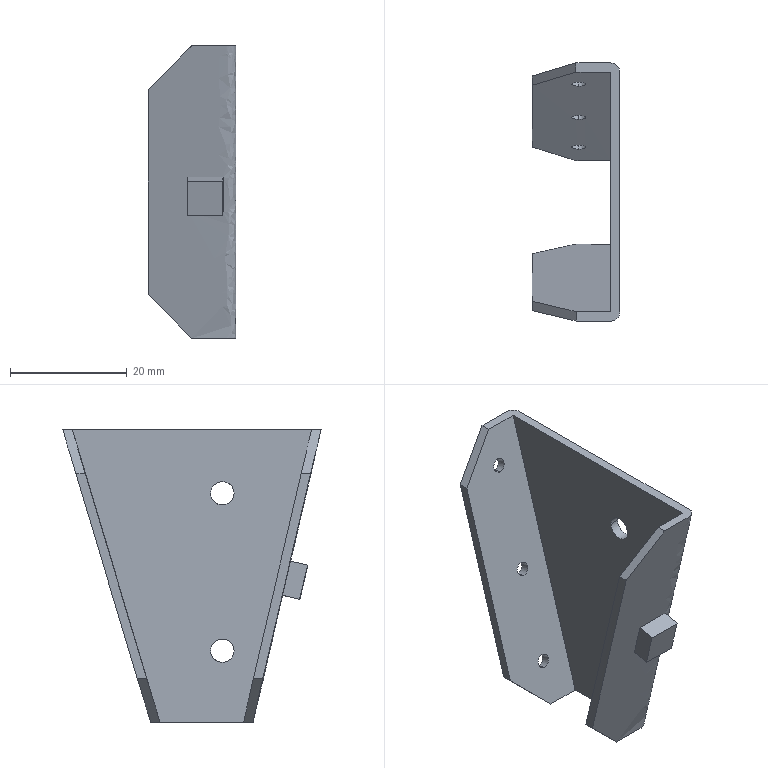Part | SolidWorks | features BaseBody 1 | 1 solid | 27 faces | box 15.009 x 44.16 x 50 mm | volume 4971 mm3 | cylinder 10 | spline 10 | plane 7 | commonest cylinder face diameters 2.4 x6 4 x4